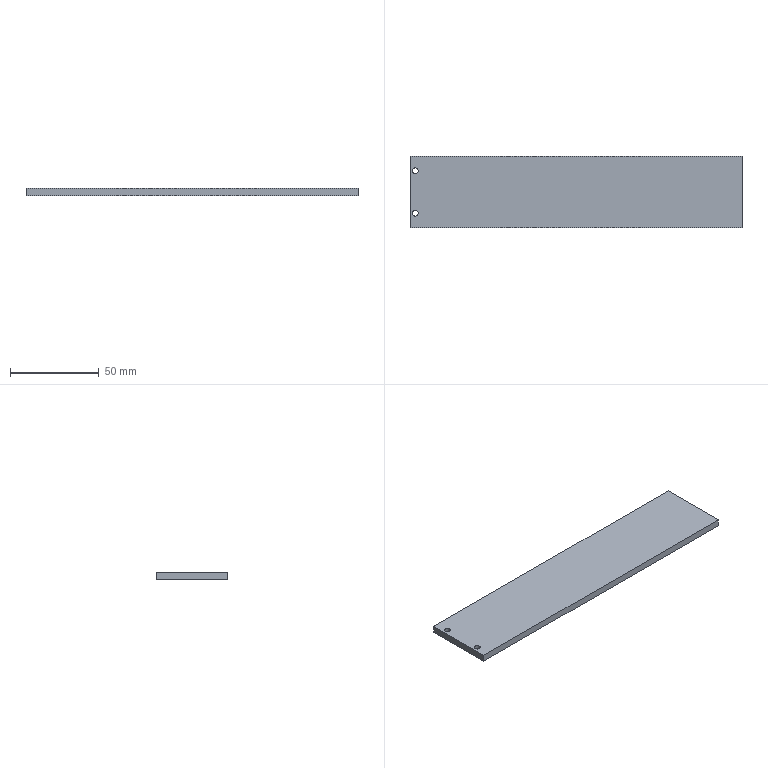Part | STEP file | Guard connecting plate | 1 solid | 10 faces | box 187 x 40 x 4 mm | volume 29852 mm3 | plane 6 | cylinder 4 | commonest cylinder face diameters 3.3 x4
STEP:
#1=CARTESIAN_POINT('',(0.,0.,0.));
#2=DIRECTION('',(0.,0.,1.));
#3=DIRECTION('',(1.,0.,0.));
#4=AXIS2_PLACEMENT_3D('',#1,#2,#3);
#5=CARTESIAN_POINT('',(-92.15,11.9,2.));
#6=VERTEX_POINT('',#5);
#7=CARTESIAN_POINT('',(-92.15,11.9,-2.));
#8=VERTEX_POINT('',#7);
#9=CARTESIAN_POINT('',(-92.15,11.9,-2.));
#10=DIRECTION('',(0.,0.,-1.));
#11=VECTOR('',#10,1.);
#12=LINE('',#9,#11);
#13=CARTESIAN_POINT('',(-90.5,11.9,-2.));
#14=DIRECTION('',(0.,0.,-1.));
#15=DIRECTION('',(-1.,0.,0.));
#16=AXIS2_PLACEMENT_3D('',#13,#14,#15);
#17=CYLINDRICAL_SURFACE('',#16,1.65);
#18=CARTESIAN_POINT('',(6.283,0.));
#19=DIRECTION('',(0.,1.));
#20=VECTOR('',#19,1.);
#21=LINE('',#18,#20);
#22=(GEOMETRIC_REPRESENTATION_CONTEXT(2)PARAMETRIC_REPRESENTATION_CONTEXT()REPRESENTATION_CONTEXT('',''));
#23=DEFINITIONAL_REPRESENTATION('',(#21),#22);
#24=PCURVE('',#17,#23);
#25=CARTESIAN_POINT('',(-90.5,11.9,-2.));
#26=DIRECTION('',(0.,0.,-1.));
#27=DIRECTION('',(-1.,0.,0.));
#28=AXIS2_PLACEMENT_3D('',#25,#26,#27);
#29=CYLINDRICAL_SURFACE('',#28,1.65);
#30=CARTESIAN_POINT('',(0.,0.));
#31=DIRECTION('',(0.,1.));
#32=VECTOR('',#31,1.);
#33=LINE('',#30,#32);
#34=(GEOMETRIC_REPRESENTATION_CONTEXT(2)PARAMETRIC_REPRESENTATION_CONTEXT()REPRESENTATION_CONTEXT('',''));
#35=DEFINITIONAL_REPRESENTATION('',(#33),#34);
#36=PCURVE('',#29,#35);
#37=SURFACE_CURVE('',#12,(#24,#36),.PCURVE_S1.);
#38=EDGE_CURVE('',#6,#8,#37,.T.);
#39=ORIENTED_EDGE('',*,*,#38,.T.);
#40=CARTESIAN_POINT('',(-88.85,11.9,-2.));
#41=VERTEX_POINT('',#40);
#42=CARTESIAN_POINT('',(-90.5,11.9,-2.));
#43=DIRECTION('',(0.,0.,-1.));
#44=DIRECTION('',(-1.,0.,0.));
#45=AXIS2_PLACEMENT_3D('',#42,#43,#44);
#46=CIRCLE('',#45,1.65);
#47=CARTESIAN_POINT('',(0.,0.));
#48=DIRECTION('',(1.,0.));
#49=VECTOR('',#48,1.);
#50=LINE('',#47,#49);
#51=(GEOMETRIC_REPRESENTATION_CONTEXT(2)PARAMETRIC_REPRESENTATION_CONTEXT()REPRESENTATION_CONTEXT('',''));
#52=DEFINITIONAL_REPRESENTATION('',(#50),#51);
#53=PCURVE('',#17,#52);
#54=CARTESIAN_POINT('',(0.,0.,-2.));
#55=DIRECTION('',(0.,0.,-1.));
#56=DIRECTION('',(-1.,0.,0.));
#57=AXIS2_PLACEMENT_3D('',#54,#55,#56);
#58=PLANE('',#57);
#59=CARTESIAN_POINT('',(90.5,11.9));
#60=DIRECTION('',(1.,0.));
#61=AXIS2_PLACEMENT_2D('',#59,#60);
#62=CIRCLE('',#61,1.65);
#63=(GEOMETRIC_REPRESENTATION_CONTEXT(2)PARAMETRIC_REPRESENTATION_CONTEXT()REPRESENTATION_CONTEXT('',''));
#64=DEFINITIONAL_REPRESENTATION('',(#62),#63);
#65=PCURVE('',#58,#64);
#66=SURFACE_CURVE('',#46,(#53,#65),.PCURVE_S1.);
#67=EDGE_CURVE('',#41,#8,#66,.T.);
#68=ORIENTED_EDGE('',*,*,#67,.F.);
#69=CARTESIAN_POINT('',(-88.85,11.9,2.));
#70=VERTEX_POINT('',#69);
#71=CARTESIAN_POINT('',(-88.85,11.9,-2.));
#72=DIRECTION('',(0.,0.,-1.));
#73=VECTOR('',#72,1.);
#74=LINE('',#71,#73);
#75=CARTESIAN_POINT('',(3.142,0.));
#76=DIRECTION('',(0.,1.));
#77=VECTOR('',#76,1.);
#78=LINE('',#75,#77);
#79=(GEOMETRIC_REPRESENTATION_CONTEXT(2)PARAMETRIC_REPRESENTATION_CONTEXT()REPRESENTATION_CONTEXT('',''));
#80=DEFINITIONAL_REPRESENTATION('',(#78),#79);
#81=PCURVE('',#17,#80);
#82=CARTESIAN_POINT('',(3.142,0.));
#83=DIRECTION('',(0.,1.));
#84=VECTOR('',#83,1.);
#85=LINE('',#82,#84);
#86=(GEOMETRIC_REPRESENTATION_CONTEXT(2)PARAMETRIC_REPRESENTATION_CONTEXT()REPRESENTATION_CONTEXT('',''));
#87=DEFINITIONAL_REPRESENTATION('',(#85),#86);
#88=PCURVE('',#29,#87);
#89=SURFACE_CURVE('',#74,(#81,#88),.PCURVE_S1.);
#90=EDGE_CURVE('',#70,#41,#89,.T.);
#91=ORIENTED_EDGE('',*,*,#90,.F.);
#92=CARTESIAN_POINT('',(-90.5,11.9,2.));
#93=DIRECTION('',(0.,0.,-1.));
#94=DIRECTION('',(-1.,0.,0.));
#95=AXIS2_PLACEMENT_3D('',#92,#93,#94);
#96=CIRCLE('',#95,1.65);
#97=CARTESIAN_POINT('',(0.,-4.));
#98=DIRECTION('',(1.,0.));
#99=VECTOR('',#98,1.);
#100=LINE('',#97,#99);
#101=(GEOMETRIC_REPRESENTATION_CONTEXT(2)PARAMETRIC_REPRESENTATION_CONTEXT()REPRESENTATION_CONTEXT('',''));
#102=DEFINITIONAL_REPRESENTATION('',(#100),#101);
#103=PCURVE('',#17,#102);
#104=CARTESIAN_POINT('',(0.,0.,2.));
#105=DIRECTION('',(0.,0.,-1.));
#106=DIRECTION('',(-1.,0.,0.));
#107=AXIS2_PLACEMENT_3D('',#104,#105,#106);
#108=PLANE('',#107);
#109=CARTESIAN_POINT('',(90.5,11.9));
#110=DIRECTION('',(1.,0.));
#111=AXIS2_PLACEMENT_2D('',#109,#110);
#112=CIRCLE('',#111,1.65);
#113=(GEOMETRIC_REPRESENTATION_CONTEXT(2)PARAMETRIC_REPRESENTATION_CONTEXT()REPRESENTATION_CONTEXT('',''));
#114=DEFINITIONAL_REPRESENTATION('',(#112),#113);
#115=PCURVE('',#108,#114);
#116=SURFACE_CURVE('',#96,(#103,#115),.PCURVE_S1.);
#117=EDGE_CURVE('',#70,#6,#116,.T.);
#118=ORIENTED_EDGE('',*,*,#117,.T.);
#119=EDGE_LOOP('',(#39,#68,#91,#118));
#120=FACE_BOUND('',#119,.F.);
#121=ADVANCED_FACE('',(#120),#17,.F.);
#122=CARTESIAN_POINT('',(-92.15,-11.9,2.));
#123=VERTEX_POINT('',#122);
#124=CARTESIAN_POINT('',(-92.15,-11.9,-2.));
#125=VERTEX_POINT('',#124);
#126=CARTESIAN_POINT('',(-92.15,-11.9,-2.));
#127=DIRECTION('',(0.,0.,-1.));
#128=VECTOR('',#127,1.);
#129=LINE('',#126,#128);
#130=CARTESIAN_POINT('',(-90.5,-11.9,-2.));
#131=DIRECTION('',(0.,0.,-1.));
#132=DIRECTION('',(-1.,0.,0.));
#133=AXIS2_PLACEMENT_3D('',#130,#131,#132);
#134=CYLINDRICAL_SURFACE('',#133,1.65);
#135=CARTESIAN_POINT('',(6.283,0.));
#136=DIRECTION('',(0.,1.));
#137=VECTOR('',#136,1.);
#138=LINE('',#135,#137);
#139=(GEOMETRIC_REPRESENTATION_CONTEXT(2)PARAMETRIC_REPRESENTATION_CONTEXT()REPRESENTATION_CONTEXT('',''));
#140=DEFINITIONAL_REPRESENTATION('',(#138),#139);
#141=PCURVE('',#134,#140);
#142=CARTESIAN_POINT('',(-90.5,-11.9,-2.));
#143=DIRECTION('',(0.,0.,-1.));
#144=DIRECTION('',(-1.,0.,0.));
#145=AXIS2_PLACEMENT_3D('',#142,#143,#144);
#146=CYLINDRICAL_SURFACE('',#145,1.65);
#147=CARTESIAN_POINT('',(0.,0.));
#148=DIRECTION('',(0.,1.));
#149=VECTOR('',#148,1.);
#150=LINE('',#147,#149);
#151=(GEOMETRIC_REPRESENTATION_CONTEXT(2)PARAMETRIC_REPRESENTATION_CONTEXT()REPRESENTATION_CONTEXT('',''));
#152=DEFINITIONAL_REPRESENTATION('',(#150),#151);
#153=PCURVE('',#146,#152);
#154=SURFACE_CURVE('',#129,(#141,#153),.PCURVE_S1.);
#155=EDGE_CURVE('',#123,#125,#154,.T.);
#156=ORIENTED_EDGE('',*,*,#155,.T.);
#157=CARTESIAN_POINT('',(-88.85,-11.9,-2.));
#158=VERTEX_POINT('',#157);
#159=CARTESIAN_POINT('',(-90.5,-11.9,-2.));
#160=DIRECTION('',(0.,0.,-1.));
#161=DIRECTION('',(-1.,0.,0.));
#162=AXIS2_PLACEMENT_3D('',#159,#160,#161);
#163=CIRCLE('',#162,1.65);
#164=CARTESIAN_POINT('',(0.,0.));
#165=DIRECTION('',(1.,0.));
#166=VECTOR('',#165,1.);
#167=LINE('',#164,#166);
#168=(GEOMETRIC_REPRESENTATION_CONTEXT(2)PARAMETRIC_REPRESENTATION_CONTEXT()REPRESENTATION_CONTEXT('',''));
#169=DEFINITIONAL_REPRESENTATION('',(#167),#168);
#170=PCURVE('',#134,#169);
#171=CARTESIAN_POINT('',(90.5,-11.9));
#172=DIRECTION('',(1.,0.));
#173=AXIS2_PLACEMENT_2D('',#171,#172);
#174=CIRCLE('',#173,1.65);
#175=(GEOMETRIC_REPRESENTATION_CONTEXT(2)PARAMETRIC_REPRESENTATION_CONTEXT()REPRESENTATION_CONTEXT('',''));
#176=DEFINITIONAL_REPRESENTATION('',(#174),#175);
#177=PCURVE('',#58,#176);
#178=SURFACE_CURVE('',#163,(#170,#177),.PCURVE_S1.);
#179=EDGE_CURVE('',#158,#125,#178,.T.);
#180=ORIENTED_EDGE('',*,*,#179,.F.);
#181=CARTESIAN_POINT('',(-88.85,-11.9,2.));
#182=VERTEX_POINT('',#181);
#183=CARTESIAN_POINT('',(-88.85,-11.9,-2.));
#184=DIRECTION('',(0.,0.,-1.));
#185=VECTOR('',#184,1.);
#186=LINE('',#183,#185);
#187=CARTESIAN_POINT('',(3.142,0.));
#188=DIRECTION('',(0.,1.));
#189=VECTOR('',#188,1.);
#190=LINE('',#187,#189);
#191=(GEOMETRIC_REPRESENTATION_CONTEXT(2)PARAMETRIC_REPRESENTATION_CONTEXT()REPRESENTATION_CONTEXT('',''));
#192=DEFINITIONAL_REPRESENTATION('',(#190),#191);
#193=PCURVE('',#134,#192);
#194=CARTESIAN_POINT('',(3.142,0.));
#195=DIRECTION('',(0.,1.));
#196=VECTOR('',#195,1.);
#197=LINE('',#194,#196);
#198=(GEOMETRIC_REPRESENTATION_CONTEXT(2)PARAMETRIC_REPRESENTATION_CONTEXT()REPRESENTATION_CONTEXT('',''));
#199=DEFINITIONAL_REPRESENTATION('',(#197),#198);
#200=PCURVE('',#146,#199);
#201=SURFACE_CURVE('',#186,(#193,#200),.PCURVE_S1.);
#202=EDGE_CURVE('',#182,#158,#201,.T.);
#203=ORIENTED_EDGE('',*,*,#202,.F.);
#204=CARTESIAN_POINT('',(-90.5,-11.9,2.));
#205=DIRECTION('',(0.,0.,-1.));
#206=DIRECTION('',(-1.,0.,0.));
#207=AXIS2_PLACEMENT_3D('',#204,#205,#206);
#208=CIRCLE('',#207,1.65);
#209=CARTESIAN_POINT('',(0.,-4.));
#210=DIRECTION('',(1.,0.));
#211=VECTOR('',#210,1.);
#212=LINE('',#209,#211);
#213=(GEOMETRIC_REPRESENTATION_CONTEXT(2)PARAMETRIC_REPRESENTATION_CONTEXT()REPRESENTATION_CONTEXT('',''));
#214=DEFINITIONAL_REPRESENTATION('',(#212),#213);
#215=PCURVE('',#134,#214);
#216=CARTESIAN_POINT('',(90.5,-11.9));
#217=DIRECTION('',(1.,0.));
#218=AXIS2_PLACEMENT_2D('',#216,#217);
#219=CIRCLE('',#218,1.65);
#220=(GEOMETRIC_REPRESENTATION_CONTEXT(2)PARAMETRIC_REPRESENTATION_CONTEXT()REPRESENTATION_CONTEXT('',''));
#221=DEFINITIONAL_REPRESENTATION('',(#219),#220);
#222=PCURVE('',#108,#221);
#223=SURFACE_CURVE('',#208,(#215,#222),.PCURVE_S1.);
#224=EDGE_CURVE('',#182,#123,#223,.T.);
#225=ORIENTED_EDGE('',*,*,#224,.T.);
#226=EDGE_LOOP('',(#156,#180,#203,#225));
#227=FACE_BOUND('',#226,.F.);
#228=ADVANCED_FACE('',(#227),#134,.F.);
#229=CARTESIAN_POINT('',(93.5,-20.,-2.));
#230=VERTEX_POINT('',#229);
#231=CARTESIAN_POINT('',(93.5,20.,-2.));
#232=VERTEX_POINT('',#231);
#233=CARTESIAN_POINT('',(93.5,-20.,-2.));
#234=DIRECTION('',(0.,1.,0.));
#235=VECTOR('',#234,1.);
#236=LINE('',#233,#235);
#237=CARTESIAN_POINT('',(93.5,-20.,2.));
#238=DIRECTION('',(-1.,0.,0.));
#239=DIRECTION('',(0.,0.,1.));
#240=AXIS2_PLACEMENT_3D('',#237,#238,#239);
#241=PLANE('',#240);
#242=CARTESIAN_POINT('',(-4.,0.));
#243=DIRECTION('',(0.,1.));
#244=VECTOR('',#243,1.);
#245=LINE('',#242,#244);
#246=(GEOMETRIC_REPRESENTATION_CONTEXT(2)PARAMETRIC_REPRESENTATION_CONTEXT()REPRESENTATION_CONTEXT('',''));
#247=DEFINITIONAL_REPRESENTATION('',(#245),#246);
#248=PCURVE('',#241,#247);
#249=CARTESIAN_POINT('',(-93.5,-20.));
#250=DIRECTION('',(0.,1.));
#251=VECTOR('',#250,1.);
#252=LINE('',#249,#251);
#253=(GEOMETRIC_REPRESENTATION_CONTEXT(2)PARAMETRIC_REPRESENTATION_CONTEXT()REPRESENTATION_CONTEXT('',''));
#254=DEFINITIONAL_REPRESENTATION('',(#252),#253);
#255=PCURVE('',#58,#254);
#256=SURFACE_CURVE('',#236,(#248,#255),.PCURVE_S1.);
#257=EDGE_CURVE('',#230,#232,#256,.T.);
#258=ORIENTED_EDGE('',*,*,#257,.T.);
#259=CARTESIAN_POINT('',(93.5,20.,2.));
#260=VERTEX_POINT('',#259);
#261=CARTESIAN_POINT('',(93.5,20.,2.));
#262=DIRECTION('',(0.,0.,-1.));
#263=VECTOR('',#262,1.);
#264=LINE('',#261,#263);
#265=CARTESIAN_POINT('',(0.,40.));
#266=DIRECTION('',(-1.,0.));
#267=VECTOR('',#266,1.);
#268=LINE('',#265,#267);
#269=(GEOMETRIC_REPRESENTATION_CONTEXT(2)PARAMETRIC_REPRESENTATION_CONTEXT()REPRESENTATION_CONTEXT('',''));
#270=DEFINITIONAL_REPRESENTATION('',(#268),#269);
#271=PCURVE('',#241,#270);
#272=CARTESIAN_POINT('',(-93.5,20.,2.));
#273=DIRECTION('',(0.,-1.,0.));
#274=DIRECTION('',(0.,0.,-1.));
#275=AXIS2_PLACEMENT_3D('',#272,#273,#274);
#276=PLANE('',#275);
#277=CARTESIAN_POINT('',(0.,187.));
#278=DIRECTION('',(1.,0.));
#279=VECTOR('',#278,1.);
#280=LINE('',#277,#279);
#281=(GEOMETRIC_REPRESENTATION_CONTEXT(2)PARAMETRIC_REPRESENTATION_CONTEXT()REPRESENTATION_CONTEXT('',''));
#282=DEFINITIONAL_REPRESENTATION('',(#280),#281);
#283=PCURVE('',#276,#282);
#284=SURFACE_CURVE('',#264,(#271,#283),.PCURVE_S1.);
#285=EDGE_CURVE('',#260,#232,#284,.T.);
#286=ORIENTED_EDGE('',*,*,#285,.F.);
#287=CARTESIAN_POINT('',(93.5,-20.,2.));
#288=VERTEX_POINT('',#287);
#289=CARTESIAN_POINT('',(93.5,-20.,2.));
#290=DIRECTION('',(0.,1.,0.));
#291=VECTOR('',#290,1.);
#292=LINE('',#289,#291);
#293=CARTESIAN_POINT('',(0.,0.));
#294=DIRECTION('',(0.,1.));
#295=VECTOR('',#294,1.);
#296=LINE('',#293,#295);
#297=(GEOMETRIC_REPRESENTATION_CONTEXT(2)PARAMETRIC_REPRESENTATION_CONTEXT()REPRESENTATION_CONTEXT('',''));
#298=DEFINITIONAL_REPRESENTATION('',(#296),#297);
#299=PCURVE('',#241,#298);
#300=CARTESIAN_POINT('',(-93.5,-20.));
#301=DIRECTION('',(0.,1.));
#302=VECTOR('',#301,1.);
#303=LINE('',#300,#302);
#304=(GEOMETRIC_REPRESENTATION_CONTEXT(2)PARAMETRIC_REPRESENTATION_CONTEXT()REPRESENTATION_CONTEXT('',''));
#305=DEFINITIONAL_REPRESENTATION('',(#303),#304);
#306=PCURVE('',#108,#305);
#307=SURFACE_CURVE('',#292,(#299,#306),.PCURVE_S1.);
#308=EDGE_CURVE('',#288,#260,#307,.T.);
#309=ORIENTED_EDGE('',*,*,#308,.F.);
#310=CARTESIAN_POINT('',(93.5,-20.,2.));
#311=DIRECTION('',(0.,0.,-1.));
#312=VECTOR('',#311,1.);
#313=LINE('',#310,#312);
#314=CARTESIAN_POINT('',(0.,0.));
#315=DIRECTION('',(-1.,0.));
#316=VECTOR('',#315,1.);
#317=LINE('',#314,#316);
#318=(GEOMETRIC_REPRESENTATION_CONTEXT(2)PARAMETRIC_REPRESENTATION_CONTEXT()REPRESENTATION_CONTEXT('',''));
#319=DEFINITIONAL_REPRESENTATION('',(#317),#318);
#320=PCURVE('',#241,#319);
#321=CARTESIAN_POINT('',(-93.5,-20.,2.));
#322=DIRECTION('',(0.,1.,0.));
#323=DIRECTION('',(0.,0.,1.));
#324=AXIS2_PLACEMENT_3D('',#321,#322,#323);
#325=PLANE('',#324);
#326=CARTESIAN_POINT('',(0.,187.));
#327=DIRECTION('',(-1.,0.));
#328=VECTOR('',#327,1.);
#329=LINE('',#326,#328);
#330=(GEOMETRIC_REPRESENTATION_CONTEXT(2)PARAMETRIC_REPRESENTATION_CONTEXT()REPRESENTATION_CONTEXT('',''));
#331=DEFINITIONAL_REPRESENTATION('',(#329),#330);
#332=PCURVE('',#325,#331);
#333=SURFACE_CURVE('',#313,(#320,#332),.PCURVE_S1.);
#334=EDGE_CURVE('',#288,#230,#333,.T.);
#335=ORIENTED_EDGE('',*,*,#334,.T.);
#336=EDGE_LOOP('',(#258,#286,#309,#335));
#337=FACE_BOUND('',#336,.T.);
#338=ADVANCED_FACE('',(#337),#241,.F.);
#339=CARTESIAN_POINT('',(-93.5,20.,-2.));
#340=VERTEX_POINT('',#339);
#341=CARTESIAN_POINT('',(-93.5,20.,-2.));
#342=DIRECTION('',(-1.,0.,0.));
#343=VECTOR('',#342,1.);
#344=LINE('',#341,#343);
#345=CARTESIAN_POINT('',(4.,0.));
#346=DIRECTION('',(0.,-1.));
#347=VECTOR('',#346,1.);
#348=LINE('',#345,#347);
#349=(GEOMETRIC_REPRESENTATION_CONTEXT(2)PARAMETRIC_REPRESENTATION_CONTEXT()REPRESENTATION_CONTEXT('',''));
#350=DEFINITIONAL_REPRESENTATION('',(#348),#349);
#351=PCURVE('',#276,#350);
#352=CARTESIAN_POINT('',(93.5,20.));
#353=DIRECTION('',(1.,0.));
#354=VECTOR('',#353,1.);
#355=LINE('',#352,#354);
#356=(GEOMETRIC_REPRESENTATION_CONTEXT(2)PARAMETRIC_REPRESENTATION_CONTEXT()REPRESENTATION_CONTEXT('',''));
#357=DEFINITIONAL_REPRESENTATION('',(#355),#356);
#358=PCURVE('',#58,#357);
#359=SURFACE_CURVE('',#344,(#351,#358),.PCURVE_S1.);
#360=EDGE_CURVE('',#232,#340,#359,.T.);
#361=ORIENTED_EDGE('',*,*,#360,.T.);
#362=CARTESIAN_POINT('',(-93.5,20.,2.));
#363=VERTEX_POINT('',#362);
#364=CARTESIAN_POINT('',(-93.5,20.,2.));
#365=DIRECTION('',(0.,0.,-1.));
#366=VECTOR('',#365,1.);
#367=LINE('',#364,#366);
#368=CARTESIAN_POINT('',(0.,0.));
#369=DIRECTION('',(1.,0.));
#370=VECTOR('',#369,1.);
#371=LINE('',#368,#370);
#372=(GEOMETRIC_REPRESENTATION_CONTEXT(2)PARAMETRIC_REPRESENTATION_CONTEXT()REPRESENTATION_CONTEXT('',''));
#373=DEFINITIONAL_REPRESENTATION('',(#371),#372);
#374=PCURVE('',#276,#373);
#375=CARTESIAN_POINT('',(-93.5,-20.,2.));
#376=DIRECTION('',(1.,0.,0.));
#377=DIRECTION('',(0.,0.,-1.));
#378=AXIS2_PLACEMENT_3D('',#375,#376,#377);
#379=PLANE('',#378);
#380=CARTESIAN_POINT('',(0.,40.));
#381=DIRECTION('',(1.,0.));
#382=VECTOR('',#381,1.);
#383=LINE('',#380,#382);
#384=(GEOMETRIC_REPRESENTATION_CONTEXT(2)PARAMETRIC_REPRESENTATION_CONTEXT()REPRESENTATION_CONTEXT('',''));
#385=DEFINITIONAL_REPRESENTATION('',(#383),#384);
#386=PCURVE('',#379,#385);
#387=SURFACE_CURVE('',#367,(#374,#386),.PCURVE_S1.);
#388=EDGE_CURVE('',#363,#340,#387,.T.);
#389=ORIENTED_EDGE('',*,*,#388,.F.);
#390=CARTESIAN_POINT('',(-93.5,20.,2.));
#391=DIRECTION('',(-1.,0.,0.));
#392=VECTOR('',#391,1.);
#393=LINE('',#390,#392);
#394=CARTESIAN_POINT('',(0.,0.));
#395=DIRECTION('',(0.,-1.));
#396=VECTOR('',#395,1.);
#397=LINE('',#394,#396);
#398=(GEOMETRIC_REPRESENTATION_CONTEXT(2)PARAMETRIC_REPRESENTATION_CONTEXT()REPRESENTATION_CONTEXT('',''));
#399=DEFINITIONAL_REPRESENTATION('',(#397),#398);
#400=PCURVE('',#276,#399);
#401=CARTESIAN_POINT('',(93.5,20.));
#402=DIRECTION('',(1.,0.));
#403=VECTOR('',#402,1.);
#404=LINE('',#401,#403);
#405=(GEOMETRIC_REPRESENTATION_CONTEXT(2)PARAMETRIC_REPRESENTATION_CONTEXT()REPRESENTATION_CONTEXT('',''));
#406=DEFINITIONAL_REPRESENTATION('',(#404),#405);
#407=PCURVE('',#108,#406);
#408=SURFACE_CURVE('',#393,(#400,#407),.PCURVE_S1.);
#409=EDGE_CURVE('',#260,#363,#408,.T.);
#410=ORIENTED_EDGE('',*,*,#409,.F.);
#411=ORIENTED_EDGE('',*,*,#285,.T.);
#412=EDGE_LOOP('',(#361,#389,#410,#411));
#413=FACE_BOUND('',#412,.T.);
#414=ADVANCED_FACE('',(#413),#276,.F.);
#415=CARTESIAN_POINT('',(-93.5,-20.,-2.));
#416=VERTEX_POINT('',#415);
#417=CARTESIAN_POINT('',(-93.5,-20.,-2.));
#418=DIRECTION('',(0.,-1.,0.));
#419=VECTOR('',#418,1.);
#420=LINE('',#417,#419);
#421=CARTESIAN_POINT('',(4.,0.));
#422=DIRECTION('',(0.,-1.));
#423=VECTOR('',#422,1.);
#424=LINE('',#421,#423);
#425=(GEOMETRIC_REPRESENTATION_CONTEXT(2)PARAMETRIC_REPRESENTATION_CONTEXT()REPRESENTATION_CONTEXT('',''));
#426=DEFINITIONAL_REPRESENTATION('',(#424),#425);
#427=PCURVE('',#379,#426);
#428=CARTESIAN_POINT('',(93.5,-20.));
#429=DIRECTION('',(0.,-1.));
#430=VECTOR('',#429,1.);
#431=LINE('',#428,#430);
#432=(GEOMETRIC_REPRESENTATION_CONTEXT(2)PARAMETRIC_REPRESENTATION_CONTEXT()REPRESENTATION_CONTEXT('',''));
#433=DEFINITIONAL_REPRESENTATION('',(#431),#432);
#434=PCURVE('',#58,#433);
#435=SURFACE_CURVE('',#420,(#427,#434),.PCURVE_S1.);
#436=EDGE_CURVE('',#340,#416,#435,.T.);
#437=ORIENTED_EDGE('',*,*,#436,.T.);
#438=CARTESIAN_POINT('',(-93.5,-20.,2.));
#439=VERTEX_POINT('',#438);
#440=CARTESIAN_POINT('',(-93.5,-20.,2.));
#441=DIRECTION('',(0.,0.,-1.));
#442=VECTOR('',#441,1.);
#443=LINE('',#440,#442);
#444=CARTESIAN_POINT('',(0.,0.));
#445=DIRECTION('',(1.,0.));
#446=VECTOR('',#445,1.);
#447=LINE('',#444,#446);
#448=(GEOMETRIC_REPRESENTATION_CONTEXT(2)PARAMETRIC_REPRESENTATION_CONTEXT()REPRESENTATION_CONTEXT('',''));
#449=DEFINITIONAL_REPRESENTATION('',(#447),#448);
#450=PCURVE('',#379,#449);
#451=CARTESIAN_POINT('',(0.,0.));
#452=DIRECTION('',(-1.,0.));
#453=VECTOR('',#452,1.);
#454=LINE('',#451,#453);
#455=(GEOMETRIC_REPRESENTATION_CONTEXT(2)PARAMETRIC_REPRESENTATION_CONTEXT()REPRESENTATION_CONTEXT('',''));
#456=DEFINITIONAL_REPRESENTATION('',(#454),#455);
#457=PCURVE('',#325,#456);
#458=SURFACE_CURVE('',#443,(#450,#457),.PCURVE_S1.);
#459=EDGE_CURVE('',#439,#416,#458,.T.);
#460=ORIENTED_EDGE('',*,*,#459,.F.);
#461=CARTESIAN_POINT('',(-93.5,-20.,2.));
#462=DIRECTION('',(0.,-1.,0.));
#463=VECTOR('',#462,1.);
#464=LINE('',#461,#463);
#465=CARTESIAN_POINT('',(0.,0.));
#466=DIRECTION('',(0.,-1.));
#467=VECTOR('',#466,1.);
#468=LINE('',#465,#467);
#469=(GEOMETRIC_REPRESENTATION_CONTEXT(2)PARAMETRIC_REPRESENTATION_CONTEXT()REPRESENTATION_CONTEXT('',''));
#470=DEFINITIONAL_REPRESENTATION('',(#468),#469);
#471=PCURVE('',#379,#470);
#472=CARTESIAN_POINT('',(93.5,-20.));
#473=DIRECTION('',(0.,-1.));
#474=VECTOR('',#473,1.);
#475=LINE('',#472,#474);
#476=(GEOMETRIC_REPRESENTATION_CONTEXT(2)PARAMETRIC_REPRESENTATION_CONTEXT()REPRESENTATION_CONTEXT('',''));
#477=DEFINITIONAL_REPRESENTATION('',(#475),#476);
#478=PCURVE('',#108,#477);
#479=SURFACE_CURVE('',#464,(#471,#478),.PCURVE_S1.);
#480=EDGE_CURVE('',#363,#439,#479,.T.);
#481=ORIENTED_EDGE('',*,*,#480,.F.);
#482=ORIENTED_EDGE('',*,*,#388,.T.);
#483=EDGE_LOOP('',(#437,#460,#481,#482));
#484=FACE_BOUND('',#483,.T.);
#485=ADVANCED_FACE('',(#484),#379,.F.);
#486=CARTESIAN_POINT('',(-93.5,-20.,-2.));
#487=DIRECTION('',(1.,0.,0.));
#488=VECTOR('',#487,1.);
#489=LINE('',#486,#488);
#490=CARTESIAN_POINT('',(-4.,0.));
#491=DIRECTION('',(0.,1.));
#492=VECTOR('',#491,1.);
#493=LINE('',#490,#492);
#494=(GEOMETRIC_REPRESENTATION_CONTEXT(2)PARAMETRIC_REPRESENTATION_CONTEXT()REPRESENTATION_CONTEXT('',''));
#495=DEFINITIONAL_REPRESENTATION('',(#493),#494);
#496=PCURVE('',#325,#495);
#497=CARTESIAN_POINT('',(93.5,-20.));
#498=DIRECTION('',(-1.,0.));
#499=VECTOR('',#498,1.);
#500=LINE('',#497,#499);
#501=(GEOMETRIC_REPRESENTATION_CONTEXT(2)PARAMETRIC_REPRESENTATION_CONTEXT()REPRESENTATION_CONTEXT('',''));
#502=DEFINITIONAL_REPRESENTATION('',(#500),#501);
#503=PCURVE('',#58,#502);
#504=SURFACE_CURVE('',#489,(#496,#503),.PCURVE_S1.);
#505=EDGE_CURVE('',#416,#230,#504,.T.);
#506=ORIENTED_EDGE('',*,*,#505,.T.);
#507=ORIENTED_EDGE('',*,*,#334,.F.);
#508=CARTESIAN_POINT('',(-93.5,-20.,2.));
#509=DIRECTION('',(1.,0.,0.));
#510=VECTOR('',#509,1.);
#511=LINE('',#508,#510);
#512=CARTESIAN_POINT('',(0.,0.));
#513=DIRECTION('',(0.,1.));
#514=VECTOR('',#513,1.);
#515=LINE('',#512,#514);
#516=(GEOMETRIC_REPRESENTATION_CONTEXT(2)PARAMETRIC_REPRESENTATION_CONTEXT()REPRESENTATION_CONTEXT('',''));
#517=DEFINITIONAL_REPRESENTATION('',(#515),#516);
#518=PCURVE('',#325,#517);
#519=CARTESIAN_POINT('',(93.5,-20.));
#520=DIRECTION('',(-1.,0.));
#521=VECTOR('',#520,1.);
#522=LINE('',#519,#521);
#523=(GEOMETRIC_REPRESENTATION_CONTEXT(2)PARAMETRIC_REPRESENTATION_CONTEXT()REPRESENTATION_CONTEXT('',''));
#524=DEFINITIONAL_REPRESENTATION('',(#522),#523);
#525=PCURVE('',#108,#524);
#526=SURFACE_CURVE('',#511,(#518,#525),.PCURVE_S1.);
#527=EDGE_CURVE('',#439,#288,#526,.T.);
#528=ORIENTED_EDGE('',*,*,#527,.F.);
#529=ORIENTED_EDGE('',*,*,#459,.T.);
#530=EDGE_LOOP('',(#506,#507,#528,#529));
#531=FACE_BOUND('',#530,.T.);
#532=ADVANCED_FACE('',(#531),#325,.F.);
#533=CARTESIAN_POINT('',(-90.5,11.9,2.));
#534=DIRECTION('',(0.,0.,-1.));
#535=DIRECTION('',(-1.,0.,0.));
#536=AXIS2_PLACEMENT_3D('',#533,#534,#535);
#537=CIRCLE('',#536,1.65);
#538=CARTESIAN_POINT('',(90.5,11.9));
#539=DIRECTION('',(1.,0.));
#540=AXIS2_PLACEMENT_2D('',#538,#539);
#541=CIRCLE('',#540,1.65);
#542=(GEOMETRIC_REPRESENTATION_CONTEXT(2)PARAMETRIC_REPRESENTATION_CONTEXT()REPRESENTATION_CONTEXT('',''));
#543=DEFINITIONAL_REPRESENTATION('',(#541),#542);
#544=PCURVE('',#108,#543);
#545=CARTESIAN_POINT('',(0.,-4.));
#546=DIRECTION('',(1.,0.));
#547=VECTOR('',#546,1.);
#548=LINE('',#545,#547);
#549=(GEOMETRIC_REPRESENTATION_CONTEXT(2)PARAMETRIC_REPRESENTATION_CONTEXT()REPRESENTATION_CONTEXT('',''));
#550=DEFINITIONAL_REPRESENTATION('',(#548),#549);
#551=PCURVE('',#29,#550);
#552=SURFACE_CURVE('',#537,(#544,#551),.PCURVE_S1.);
#553=EDGE_CURVE('',#6,#70,#552,.T.);
#554=ORIENTED_EDGE('',*,*,#553,.T.);
#555=ORIENTED_EDGE('',*,*,#117,.T.);
#556=EDGE_LOOP('',(#554,#555));
#557=FACE_BOUND('',#556,.T.);
#558=CARTESIAN_POINT('',(-90.5,-11.9,2.));
#559=DIRECTION('',(0.,0.,-1.));
#560=DIRECTION('',(-1.,0.,0.));
#561=AXIS2_PLACEMENT_3D('',#558,#559,#560);
#562=CIRCLE('',#561,1.65);
#563=CARTESIAN_POINT('',(90.5,-11.9));
#564=DIRECTION('',(1.,0.));
#565=AXIS2_PLACEMENT_2D('',#563,#564);
#566=CIRCLE('',#565,1.65);
#567=(GEOMETRIC_REPRESENTATION_CONTEXT(2)PARAMETRIC_REPRESENTATION_CONTEXT()REPRESENTATION_CONTEXT('',''));
#568=DEFINITIONAL_REPRESENTATION('',(#566),#567);
#569=PCURVE('',#108,#568);
#570=CARTESIAN_POINT('',(0.,-4.));
#571=DIRECTION('',(1.,0.));
#572=VECTOR('',#571,1.);
#573=LINE('',#570,#572);
#574=(GEOMETRIC_REPRESENTATION_CONTEXT(2)PARAMETRIC_REPRESENTATION_CONTEXT()REPRESENTATION_CONTEXT('',''));
#575=DEFINITIONAL_REPRESENTATION('',(#573),#574);
#576=PCURVE('',#146,#575);
#577=SURFACE_CURVE('',#562,(#569,#576),.PCURVE_S1.);
#578=EDGE_CURVE('',#123,#182,#577,.T.);
#579=ORIENTED_EDGE('',*,*,#578,.T.);
#580=ORIENTED_EDGE('',*,*,#224,.T.);
#581=EDGE_LOOP('',(#579,#580));
#582=FACE_BOUND('',#581,.T.);
#583=ORIENTED_EDGE('',*,*,#308,.T.);
#584=ORIENTED_EDGE('',*,*,#409,.T.);
#585=ORIENTED_EDGE('',*,*,#480,.T.);
#586=ORIENTED_EDGE('',*,*,#527,.T.);
#587=EDGE_LOOP('',(#583,#584,#585,#586));
#588=FACE_BOUND('',#587,.T.);
#589=ADVANCED_FACE('',(#557,#582,#588),#108,.F.);
#590=CARTESIAN_POINT('',(-90.5,11.9,-2.));
#591=DIRECTION('',(0.,0.,-1.));
#592=DIRECTION('',(-1.,0.,0.));
#593=AXIS2_PLACEMENT_3D('',#590,#591,#592);
#594=CIRCLE('',#593,1.65);
#595=CARTESIAN_POINT('',(90.5,11.9));
#596=DIRECTION('',(1.,0.));
#597=AXIS2_PLACEMENT_2D('',#595,#596);
#598=CIRCLE('',#597,1.65);
#599=(GEOMETRIC_REPRESENTATION_CONTEXT(2)PARAMETRIC_REPRESENTATION_CONTEXT()REPRESENTATION_CONTEXT('',''));
#600=DEFINITIONAL_REPRESENTATION('',(#598),#599);
#601=PCURVE('',#58,#600);
#602=CARTESIAN_POINT('',(0.,0.));
#603=DIRECTION('',(1.,0.));
#604=VECTOR('',#603,1.);
#605=LINE('',#602,#604);
#606=(GEOMETRIC_REPRESENTATION_CONTEXT(2)PARAMETRIC_REPRESENTATION_CONTEXT()REPRESENTATION_CONTEXT('',''));
#607=DEFINITIONAL_REPRESENTATION('',(#605),#606);
#608=PCURVE('',#29,#607);
#609=SURFACE_CURVE('',#594,(#601,#608),.PCURVE_S1.);
#610=EDGE_CURVE('',#8,#41,#609,.T.);
#611=ORIENTED_EDGE('',*,*,#610,.F.);
#612=ORIENTED_EDGE('',*,*,#67,.F.);
#613=EDGE_LOOP('',(#611,#612));
#614=FACE_BOUND('',#613,.T.);
#615=CARTESIAN_POINT('',(-90.5,-11.9,-2.));
#616=DIRECTION('',(0.,0.,-1.));
#617=DIRECTION('',(-1.,0.,0.));
#618=AXIS2_PLACEMENT_3D('',#615,#616,#617);
#619=CIRCLE('',#618,1.65);
#620=CARTESIAN_POINT('',(90.5,-11.9));
#621=DIRECTION('',(1.,0.));
#622=AXIS2_PLACEMENT_2D('',#620,#621);
#623=CIRCLE('',#622,1.65);
#624=(GEOMETRIC_REPRESENTATION_CONTEXT(2)PARAMETRIC_REPRESENTATION_CONTEXT()REPRESENTATION_CONTEXT('',''));
#625=DEFINITIONAL_REPRESENTATION('',(#623),#624);
#626=PCURVE('',#58,#625);
#627=CARTESIAN_POINT('',(0.,0.));
#628=DIRECTION('',(1.,0.));
#629=VECTOR('',#628,1.);
#630=LINE('',#627,#629);
#631=(GEOMETRIC_REPRESENTATION_CONTEXT(2)PARAMETRIC_REPRESENTATION_CONTEXT()REPRESENTATION_CONTEXT('',''));
#632=DEFINITIONAL_REPRESENTATION('',(#630),#631);
#633=PCURVE('',#146,#632);
#634=SURFACE_CURVE('',#619,(#626,#633),.PCURVE_S1.);
#635=EDGE_CURVE('',#125,#158,#634,.T.);
#636=ORIENTED_EDGE('',*,*,#635,.F.);
#637=ORIENTED_EDGE('',*,*,#179,.F.);
#638=EDGE_LOOP('',(#636,#637));
#639=FACE_BOUND('',#638,.T.);
#640=ORIENTED_EDGE('',*,*,#257,.F.);
#641=ORIENTED_EDGE('',*,*,#505,.F.);
#642=ORIENTED_EDGE('',*,*,#436,.F.);
#643=ORIENTED_EDGE('',*,*,#360,.F.);
#644=EDGE_LOOP('',(#640,#641,#642,#643));
#645=FACE_BOUND('',#644,.T.);
#646=ADVANCED_FACE('',(#614,#639,#645),#58,.T.);
#647=ORIENTED_EDGE('',*,*,#635,.F.);
#648=ORIENTED_EDGE('',*,*,#155,.F.);
#649=ORIENTED_EDGE('',*,*,#578,.T.);
#650=ORIENTED_EDGE('',*,*,#202,.T.);
#651=EDGE_LOOP('',(#647,#648,#649,#650));
#652=FACE_BOUND('',#651,.F.);
#653=ADVANCED_FACE('',(#652),#146,.F.);
#654=ORIENTED_EDGE('',*,*,#610,.F.);
#655=ORIENTED_EDGE('',*,*,#38,.F.);
#656=ORIENTED_EDGE('',*,*,#553,.T.);
#657=ORIENTED_EDGE('',*,*,#90,.T.);
#658=EDGE_LOOP('',(#654,#655,#656,#657));
#659=FACE_BOUND('',#658,.F.);
#660=ADVANCED_FACE('',(#659),#29,.F.);
#661=CLOSED_SHELL('',(#121,#228,#338,#414,#485,#532,#589,#646,#653,#660));
#662=MANIFOLD_SOLID_BREP('',#661);
#663=(LENGTH_UNIT()NAMED_UNIT(*)SI_UNIT(.MILLI.,.METRE.));
#664=UNCERTAINTY_MEASURE_WITH_UNIT(LENGTH_MEASURE(0.0000001),#663,'','');
#665=(NAMED_UNIT(*)PLANE_ANGLE_UNIT()SI_UNIT($,.RADIAN.));
#666=(NAMED_UNIT(*)SI_UNIT($,.STERADIAN.)SOLID_ANGLE_UNIT());
#667=(GEOMETRIC_REPRESENTATION_CONTEXT(3)GLOBAL_UNCERTAINTY_ASSIGNED_CONTEXT((#664))GLOBAL_UNIT_ASSIGNED_CONTEXT((#663,#665,#666))REPRESENTATION_CONTEXT('',''));
#668=ADVANCED_BREP_SHAPE_REPRESENTATION('',(#4,#662),#667);